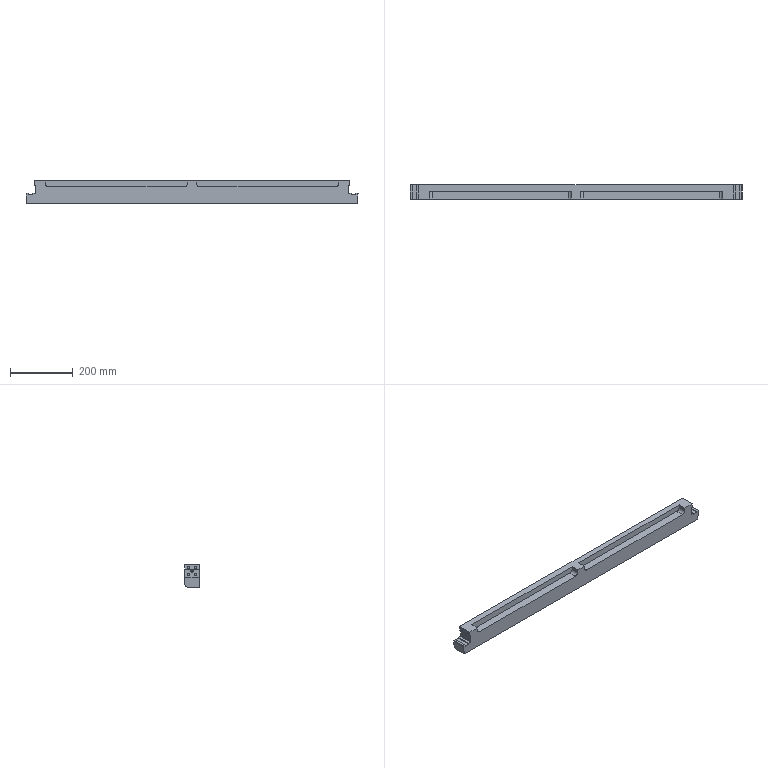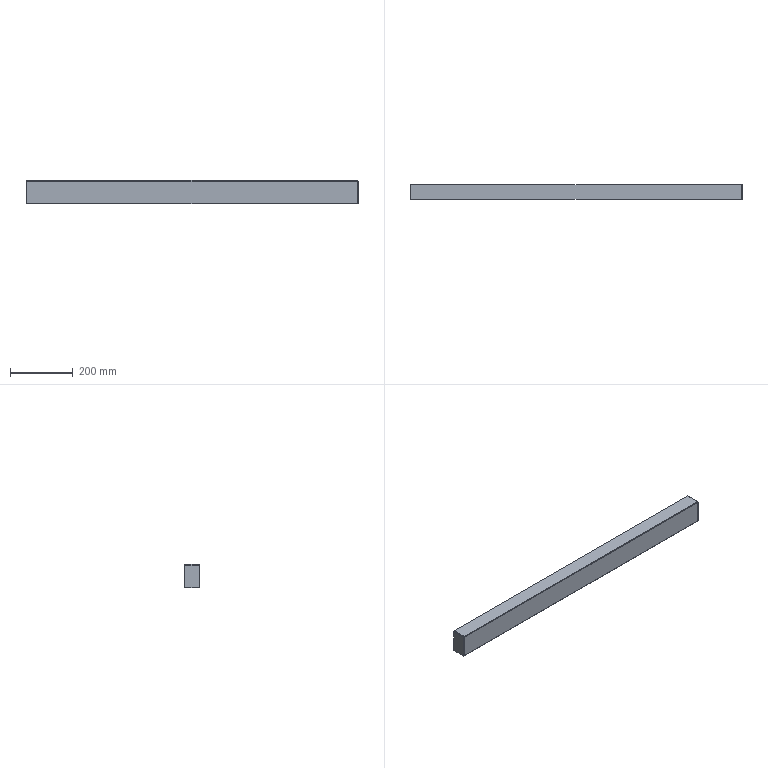CAM job | NX | 3+2 milling | part box 1056 x 45 x 72.5 mm | stock box 1062 x 45 x 75.5 mm
Tools:
number,name,description,diameter,corner_radius,flute_length,length,flutes
5,D50,Milling Tool-5 Parameters,50.0,0.0,50.0,105.0,2
21,D12JING,Milling Tool-5 Parameters,12.0,0.0,50.0,75.0,2
23,T50H10,Milling Tool-T Cutter,50.0,,10.0,25.0,4
7,D10A45,Milling Tool-5 Parameters,10.0,0.0,5.0,5.0,2
20,D12,Milling Tool-5 Parameters,12.0,0.0,50.0,75.0,2
10,D10,Milling Tool-5 Parameters,10.0,0.0,50.0,75.0,2
11,D10JING,Milling Tool-5 Parameters,10.0,0.0,50.0,75.0,2
9,D30内R刀,User Defined Mill Tool,0.0,,10.0,54.0,2
Operations:
program,operation,operation_type,tool,method,geometry_group,spindle_rpm,surface_speed,feed_per_tooth,feed_cut,feed_plunge,cut_length_mm,path_length_mm,cut_time_min,machine_time_min
1,ZLEVEL_PROFILE,ZLevelMilling,D50,METHOD,A,6500.0,1021.0,0.1538,2000.0,100.0,4638.55,5940.439,2.319,2.45
1,FLOOR_WALL_COPY_COPY,VolumeBased25DMillingOperation,D50,METHOD,A,6500.0,1286.0,0.0962,1250.0,100.0,214.8,1465,0.1718,0.2969
1,ZLEVEL_PROFILE_COPY_2,ZLevelMilling,D50,METHOD,MCS_MILL-A,6500.0,1021.0,0.1538,2000.0,100.0,2156.752,2236.952,1.078,1.086
1,ZLEVEL_PROFILE_COPY,ZLevelMilling,D12JING,METHOD,A,6500.0,326.0,0.1538,2000.0,100.0,1064.661,2675.192,0.5323,0.6934
1,刀补9,ZLevelMilling,D12JING,METHOD,A,6500.0,326.0,0.0769,1000.0,100.0,131.779,1280.428,0.1318,0.2466
1,刀补9.,ZLevelMilling,D12JING,METHOD,A,6500.0,326.0,0.0769,1000.0,100.0,274.773,1743.821,0.2748,0.4217
1,PLANAR_MILL,PlanarMilling,T50H10,METHOD,A,6000.0,942.0,0.0521,1250.0,100.0,4290.17,5767.439,2.28,2.428
1,PLANAR_MILL_1,PlanarMilling,D10A45,METHOD,A,7500.0,141.0,0.0833,1250.0,100.0,2103.442,2119.442,1.683,1.684
1,ZLEVEL_PROFILE_1_COPY_1_COPY_COPY_1_COPY,ZLevelMilling,D10A45,METHOD,A,7000.0,219.0,0.0714,1000.0,100.0,270.704,1735.836,0.2707,0.4172
2,ZLEVEL_PROFILE_COPY_1,ZLevelMilling,D12,METHOD,B,7500.0,235.0,0.2,3000.0,100.0,4551.355,5924.156,1.517,1.654
2,111,ZLevelMilling,D12JING,METHOD,B,6500.0,326.0,0.0769,1000.0,100.0,383.721,2370.025,0.3837,0.5824
2,FLOOR_WALL_1,VolumeBased25DMillingOperation,D10,METHOD,B,7500.0,0.0,0.0,3000.0,1000.0,22172.844,23290.091,7.399,7.511
2,FLOOR_WALL_2,VolumeBased25DMillingOperation,D10JING,METHOD,B,7000.0,219.0,0.0893,1250.0,100.0,4542.787,5953.158,3.634,3.775
2,ZLEVEL_PROFILE_1_COPY_1_COPY_COPY_1_COPY_COPY,ZLevelMilling,D10A45,METHOD,B,7000.0,219.0,0.0714,1000.0,100.0,2346.66,2407.66,2.347,2.353
2,ZLEVEL_PROFILE_1_COPY_1_COPY_COPY_1_COPY_COPY_COPY,ZLevelMilling,D10A45,METHOD,B,7000.0,219.0,0.0714,1000.0,100.0,906.039,2062.32,0.906,1.022
3,ZLEVEL_PROFILE_2,ZLevelMilling,D12,METHOD,C,7500.0,282.0,0.2,3000.0,1001.0,19978.818,20847.697,6.747,6.834
3,11,ZLevelMilling,D12,METHOD,C,6500.0,326.0,0.0769,1000.0,100.0,1801.604,2538.224,1.802,1.875
3,ZLEVEL_PROFILE_1_COPY_1_COPY_COPY_1_COPY_1_COPY_1,ZLevelMilling,D10A45,METHOD,C,7500.0,141.0,0.0667,1000.0,100.0,1863.044,2522.644,1.863,1.929
3,ZLEVEL_PROFILE_1_COPY_1_COPY_COPY_1_COPY_COPY_1,ZLevelMilling,D10A45,METHOD,C,7000.0,219.0,0.0714,1000.0,100.0,260.023,1387.691,0.26,0.3728
3,PLANAR_PROFILE_COPY_COPY_COPY,PlanarMilling,D30内R刀,METHOD,C,7500.0,0.0,0.0,1250.0,100.0,1071.909,1145.909,0.8575,0.8649
3,PLANAR_PROFILE_COPY_COPY_COPY_COPY,PlanarMilling,D30内R刀,METHOD,C,7500.0,0.0,0.0,1250.0,100.0,1071.909,1145.909,0.8575,0.8649
3,PLANAR_PROFILE_COPY_COPY_COPY_COPY_COPY,PlanarMilling,D30内R刀,METHOD,C,7500.0,0.0,0.0,1250.0,100.0,1071.909,1145.909,0.8575,0.8649
3,PLANAR_PROFILE_COPY_COPY_COPY_COPY_COPY_COPY,PlanarMilling,D30内R刀,METHOD,C,7500.0,0.0,0.0,1250.0,100.0,1071.909,1145.909,0.8575,0.8649